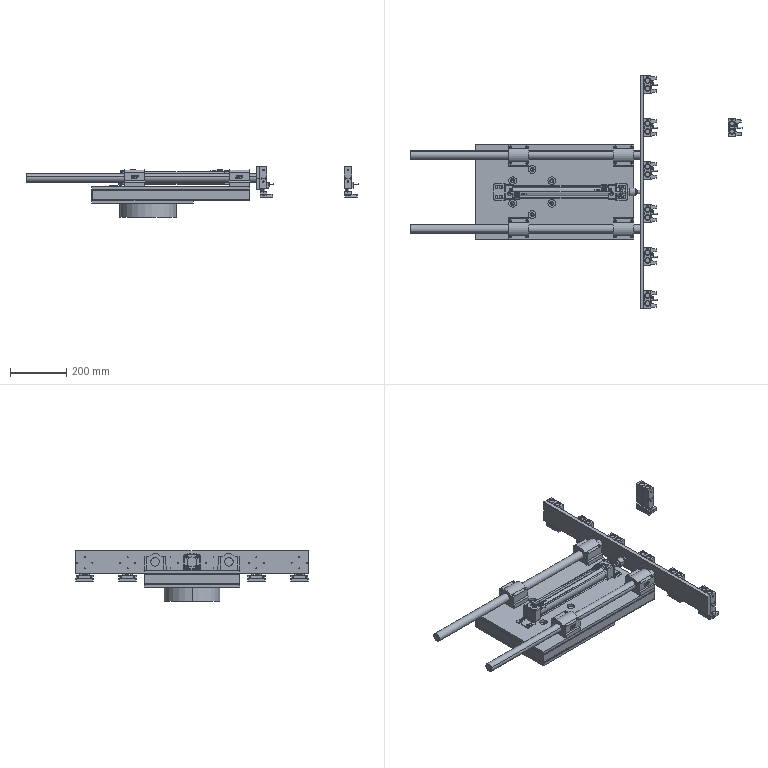Part | SolidWorks | 57 solids | 5024 faces | volume 9355579 mm3 | plane 2358 | cylinder 1554 | cone 578 | spline 496 | torus 38 | commonest cylinder face diameters 0.4 x218 20 x128 4.5 x98 10 x94 3.242 x92 4 x84